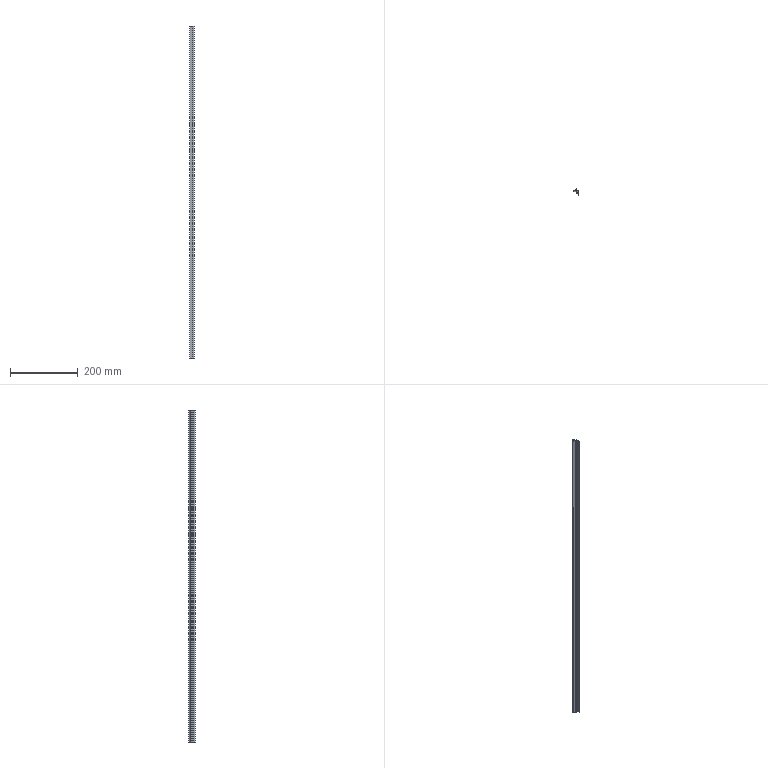Part | SolidWorks | features BaseBody 1, ICE 1, MoveFace 1 | 1 solid | 27 faces | box 14 x 20.3 x 980 mm | volume 49897 mm3 | plane 20 | cylinder 7 | commonest cylinder face diameters 0.387 x2 0.8 x2 0.4 x1 20 x1 22 x1
STEP:
#1=CARTESIAN_POINT('',(-5.304,-0.625,200.));
#2=VERTEX_POINT('',#1);
#3=CARTESIAN_POINT('',(-5.449,-0.8125,200.));
#4=VERTEX_POINT('',#3);
#5=CARTESIAN_POINT('',(-5.255,-0.8125,200.));
#6=DIRECTION('',(0.,0.,1.));
#7=DIRECTION('',(-1.,0.,0.));
#8=AXIS2_PLACEMENT_3D('',#5,#6,#7);
#9=CIRCLE('',#8,0.1937);
#10=EDGE_CURVE('',#2,#4,#9,.T.);
#11=ORIENTED_EDGE('',*,*,#10,.T.);
#12=CARTESIAN_POINT('',(-5.449,-0.8125,-780.));
#13=VERTEX_POINT('',#12);
#14=CARTESIAN_POINT('',(-5.449,-0.8125,230.));
#15=DIRECTION('',(0.,0.,-1.));
#16=VECTOR('',#15,1000.);
#17=LINE('',#14,#16);
#18=EDGE_CURVE('',#4,#13,#17,.T.);
#19=ORIENTED_EDGE('',*,*,#18,.T.);
#20=CARTESIAN_POINT('',(-5.304,-0.625,-780.));
#21=VERTEX_POINT('',#20);
#22=CARTESIAN_POINT('',(-5.255,-0.8125,-780.));
#23=DIRECTION('',(0.,0.,-1.));
#24=DIRECTION('',(1.,0.,0.));
#25=AXIS2_PLACEMENT_3D('',#22,#23,#24);
#26=CIRCLE('',#25,0.1937);
#27=EDGE_CURVE('',#13,#21,#26,.T.);
#28=ORIENTED_EDGE('',*,*,#27,.T.);
#29=CARTESIAN_POINT('',(-5.304,-0.625,230.));
#30=DIRECTION('',(0.,0.,-1.));
#31=VECTOR('',#30,1000.);
#32=LINE('',#29,#31);
#33=EDGE_CURVE('',#2,#21,#32,.T.);
#34=ORIENTED_EDGE('',*,*,#33,.F.);
#35=EDGE_LOOP('',(#11,#19,#28,#34));
#36=FACE_OUTER_BOUND('',#35,.T.);
#37=CARTESIAN_POINT('',(-5.255,-0.8125,230.));
#38=DIRECTION('',(0.,0.,-1.));
#39=DIRECTION('',(-1.,0.,0.));
#40=AXIS2_PLACEMENT_3D('',#37,#38,#39);
#41=CYLINDRICAL_SURFACE('',#40,0.1937);
#42=ADVANCED_FACE('',(#36),#41,.F.);
#43=CARTESIAN_POINT('',(5.,-1.,-780.));
#44=VERTEX_POINT('',#43);
#45=CARTESIAN_POINT('',(5.,-14.3,-780.));
#46=VERTEX_POINT('',#45);
#47=CARTESIAN_POINT('',(5.,29.623,-780.));
#48=DIRECTION('',(0.,-1.,0.));
#49=VECTOR('',#48,1000.);
#50=LINE('',#47,#49);
#51=EDGE_CURVE('',#44,#46,#50,.T.);
#52=ORIENTED_EDGE('',*,*,#51,.F.);
#53=CARTESIAN_POINT('',(5.,-1.,200.));
#54=VERTEX_POINT('',#53);
#55=CARTESIAN_POINT('',(5.,-1.,230.));
#56=DIRECTION('',(0.,0.,-1.));
#57=VECTOR('',#56,1000.);
#58=LINE('',#55,#57);
#59=EDGE_CURVE('',#54,#44,#58,.T.);
#60=ORIENTED_EDGE('',*,*,#59,.F.);
#61=CARTESIAN_POINT('',(5.,-14.3,200.));
#62=VERTEX_POINT('',#61);
#63=CARTESIAN_POINT('',(5.,-14.3,200.));
#64=DIRECTION('',(0.,1.,0.));
#65=VECTOR('',#64,1000.);
#66=LINE('',#63,#65);
#67=EDGE_CURVE('',#62,#54,#66,.T.);
#68=ORIENTED_EDGE('',*,*,#67,.F.);
#69=CARTESIAN_POINT('',(5.,-14.3,230.));
#70=DIRECTION('',(0.,0.,1.));
#71=VECTOR('',#70,1000.);
#72=LINE('',#69,#71);
#73=EDGE_CURVE('',#46,#62,#72,.T.);
#74=ORIENTED_EDGE('',*,*,#73,.F.);
#75=EDGE_LOOP('',(#52,#60,#68,#74));
#76=FACE_OUTER_BOUND('',#75,.T.);
#77=CARTESIAN_POINT('',(5.,-14.3,230.));
#78=DIRECTION('',(-1.,0.,0.));
#79=DIRECTION('',(0.,0.,1.));
#80=AXIS2_PLACEMENT_3D('',#77,#78,#79);
#81=PLANE('',#80);
#82=ADVANCED_FACE('',(#76),#81,.F.);
#83=CARTESIAN_POINT('',(-9.,-2.,-780.));
#84=VERTEX_POINT('',#83);
#85=CARTESIAN_POINT('',(-9.,-2.,200.));
#86=VERTEX_POINT('',#85);
#87=CARTESIAN_POINT('',(-9.,-2.,230.));
#88=DIRECTION('',(0.,0.,1.));
#89=VECTOR('',#88,1000.);
#90=LINE('',#87,#89);
#91=EDGE_CURVE('',#84,#86,#90,.T.);
#92=ORIENTED_EDGE('',*,*,#91,.F.);
#93=CARTESIAN_POINT('',(0.9,-2.,-780.));
#94=VERTEX_POINT('',#93);
#95=CARTESIAN_POINT('',(5.,-2.,-780.));
#96=DIRECTION('',(-1.,0.,0.));
#97=VECTOR('',#96,1000.);
#98=LINE('',#95,#97);
#99=EDGE_CURVE('',#94,#84,#98,.T.);
#100=ORIENTED_EDGE('',*,*,#99,.F.);
#101=CARTESIAN_POINT('',(0.9,-2.,200.));
#102=VERTEX_POINT('',#101);
#103=CARTESIAN_POINT('',(0.9,-2.,230.));
#104=DIRECTION('',(0.,0.,-1.));
#105=VECTOR('',#104,1000.);
#106=LINE('',#103,#105);
#107=EDGE_CURVE('',#102,#94,#106,.T.);
#108=ORIENTED_EDGE('',*,*,#107,.F.);
#109=CARTESIAN_POINT('',(5.,-2.,200.));
#110=DIRECTION('',(1.,0.,0.));
#111=VECTOR('',#110,1000.);
#112=LINE('',#109,#111);
#113=EDGE_CURVE('',#86,#102,#112,.T.);
#114=ORIENTED_EDGE('',*,*,#113,.F.);
#115=EDGE_LOOP('',(#92,#100,#108,#114));
#116=FACE_OUTER_BOUND('',#115,.T.);
#117=CARTESIAN_POINT('',(-9.,-2.,230.));
#118=DIRECTION('',(0.,1.,0.));
#119=DIRECTION('',(0.,0.,1.));
#120=AXIS2_PLACEMENT_3D('',#117,#118,#119);
#121=PLANE('',#120);
#122=ADVANCED_FACE('',(#116),#121,.F.);
#123=CARTESIAN_POINT('',(4.,-6.,200.));
#124=VERTEX_POINT('',#123);
#125=CARTESIAN_POINT('',(4.,-3.,200.));
#126=VERTEX_POINT('',#125);
#127=CARTESIAN_POINT('',(4.,29.623,200.));
#128=DIRECTION('',(0.,1.,0.));
#129=VECTOR('',#128,1000.);
#130=LINE('',#127,#129);
#131=EDGE_CURVE('',#124,#126,#130,.T.);
#132=ORIENTED_EDGE('',*,*,#131,.F.);
#133=CARTESIAN_POINT('',(1.,-6.,200.));
#134=VERTEX_POINT('',#133);
#135=CARTESIAN_POINT('',(5.,-6.,200.));
#136=DIRECTION('',(1.,0.,0.));
#137=VECTOR('',#136,1000.);
#138=LINE('',#135,#137);
#139=EDGE_CURVE('',#134,#124,#138,.T.);
#140=ORIENTED_EDGE('',*,*,#139,.F.);
#141=CARTESIAN_POINT('',(1.,-6.7,200.));
#142=VERTEX_POINT('',#141);
#143=CARTESIAN_POINT('',(1.,-6.,200.));
#144=DIRECTION('',(0.,-1.,0.));
#145=VECTOR('',#144,1000.);
#146=LINE('',#143,#145);
#147=EDGE_CURVE('',#134,#142,#146,.T.);
#148=ORIENTED_EDGE('',*,*,#147,.T.);
#149=CARTESIAN_POINT('',(-1.7,-6.7,200.));
#150=VERTEX_POINT('',#149);
#151=CARTESIAN_POINT('',(5.,-6.7,200.));
#152=DIRECTION('',(1.,0.,0.));
#153=VECTOR('',#152,1000.);
#154=LINE('',#151,#153);
#155=EDGE_CURVE('',#150,#142,#154,.T.);
#156=ORIENTED_EDGE('',*,*,#155,.F.);
#157=CARTESIAN_POINT('',(-1.7,-7.7,200.));
#158=VERTEX_POINT('',#157);
#159=CARTESIAN_POINT('',(-1.7,-6.7,200.));
#160=DIRECTION('',(0.,-1.,0.));
#161=VECTOR('',#160,1000.);
#162=LINE('',#159,#161);
#163=EDGE_CURVE('',#150,#158,#162,.T.);
#164=ORIENTED_EDGE('',*,*,#163,.T.);
#165=CARTESIAN_POINT('',(4.,-7.7,200.));
#166=VERTEX_POINT('',#165);
#167=CARTESIAN_POINT('',(5.,-7.7,200.));
#168=DIRECTION('',(-1.,0.,0.));
#169=VECTOR('',#168,1000.);
#170=LINE('',#167,#169);
#171=EDGE_CURVE('',#166,#158,#170,.T.);
#172=ORIENTED_EDGE('',*,*,#171,.F.);
#173=CARTESIAN_POINT('',(4.,-14.3,200.));
#174=VERTEX_POINT('',#173);
#175=CARTESIAN_POINT('',(4.,29.623,200.));
#176=DIRECTION('',(0.,1.,0.));
#177=VECTOR('',#176,1000.);
#178=LINE('',#175,#177);
#179=EDGE_CURVE('',#174,#166,#178,.T.);
#180=ORIENTED_EDGE('',*,*,#179,.F.);
#181=CARTESIAN_POINT('',(5.,-14.3,200.));
#182=DIRECTION('',(-1.,0.,0.));
#183=VECTOR('',#182,1000.);
#184=LINE('',#181,#183);
#185=EDGE_CURVE('',#62,#174,#184,.T.);
#186=ORIENTED_EDGE('',*,*,#185,.F.);
#187=ORIENTED_EDGE('',*,*,#67,.T.);
#188=CARTESIAN_POINT('',(-5.207,-1.,200.));
#189=VERTEX_POINT('',#188);
#190=CARTESIAN_POINT('',(5.,-1.,200.));
#191=DIRECTION('',(1.,0.,0.));
#192=VECTOR('',#191,1000.);
#193=LINE('',#190,#192);
#194=EDGE_CURVE('',#189,#54,#193,.T.);
#195=ORIENTED_EDGE('',*,*,#194,.F.);
#196=CARTESIAN_POINT('',(-5.255,-0.8125,200.));
#197=DIRECTION('',(0.,0.,1.));
#198=DIRECTION('',(-1.,0.,0.));
#199=AXIS2_PLACEMENT_3D('',#196,#197,#198);
#200=CIRCLE('',#199,0.1937);
#201=EDGE_CURVE('',#4,#189,#200,.T.);
#202=ORIENTED_EDGE('',*,*,#201,.F.);
#203=ORIENTED_EDGE('',*,*,#10,.F.);
#204=CARTESIAN_POINT('',(-1.368,3.063,200.));
#205=VERTEX_POINT('',#204);
#206=CARTESIAN_POINT('',(-10.628,9.,200.));
#207=DIRECTION('',(0.,0.,1.));
#208=DIRECTION('',(-1.,0.,0.));
#209=AXIS2_PLACEMENT_3D('',#206,#207,#208);
#210=CIRCLE('',#209,11.);
#211=EDGE_CURVE('',#2,#205,#210,.T.);
#212=ORIENTED_EDGE('',*,*,#211,.T.);
#213=CARTESIAN_POINT('',(-1.,2.955,200.));
#214=VERTEX_POINT('',#213);
#215=CARTESIAN_POINT('',(-1.2,2.955,200.));
#216=DIRECTION('',(0.,0.,1.));
#217=DIRECTION('',(-1.,0.,0.));
#218=AXIS2_PLACEMENT_3D('',#215,#216,#217);
#219=CIRCLE('',#218,0.2);
#220=EDGE_CURVE('',#214,#205,#219,.T.);
#221=ORIENTED_EDGE('',*,*,#220,.F.);
#222=CARTESIAN_POINT('',(-1.,1.5,200.));
#223=VERTEX_POINT('',#222);
#224=CARTESIAN_POINT('',(-1.,2.955,200.));
#225=DIRECTION('',(0.,1.,0.));
#226=VECTOR('',#225,1000.);
#227=LINE('',#224,#226);
#228=EDGE_CURVE('',#223,#214,#227,.T.);
#229=ORIENTED_EDGE('',*,*,#228,.F.);
#230=CARTESIAN_POINT('',(0.,1.5,200.));
#231=VERTEX_POINT('',#230);
#232=CARTESIAN_POINT('',(-1.,1.5,200.));
#233=DIRECTION('',(-1.,0.,0.));
#234=VECTOR('',#233,1000.);
#235=LINE('',#232,#234);
#236=EDGE_CURVE('',#231,#223,#235,.T.);
#237=ORIENTED_EDGE('',*,*,#236,.F.);
#238=CARTESIAN_POINT('',(0.,6.,200.));
#239=VERTEX_POINT('',#238);
#240=CARTESIAN_POINT('',(0.,1.5,200.));
#241=DIRECTION('',(0.,-1.,0.));
#242=VECTOR('',#241,1000.);
#243=LINE('',#240,#242);
#244=EDGE_CURVE('',#239,#231,#243,.T.);
#245=ORIENTED_EDGE('',*,*,#244,.F.);
#246=CARTESIAN_POINT('',(-0.8,6.,200.));
#247=VERTEX_POINT('',#246);
#248=CARTESIAN_POINT('',(0.,6.,200.));
#249=DIRECTION('',(1.,0.,0.));
#250=VECTOR('',#249,1000.);
#251=LINE('',#248,#250);
#252=EDGE_CURVE('',#247,#239,#251,.T.);
#253=ORIENTED_EDGE('',*,*,#252,.F.);
#254=CARTESIAN_POINT('',(-1.178,5.731,200.));
#255=VERTEX_POINT('',#254);
#256=CARTESIAN_POINT('',(-0.8,5.6,200.));
#257=DIRECTION('',(0.,0.,1.));
#258=DIRECTION('',(-1.,0.,0.));
#259=AXIS2_PLACEMENT_3D('',#256,#257,#258);
#260=CIRCLE('',#259,0.4);
#261=EDGE_CURVE('',#247,#255,#260,.T.);
#262=ORIENTED_EDGE('',*,*,#261,.T.);
#263=CARTESIAN_POINT('',(-8.678,-0.8077,200.));
#264=VERTEX_POINT('',#263);
#265=CARTESIAN_POINT('',(-10.628,9.,200.));
#266=DIRECTION('',(0.,0.,1.));
#267=DIRECTION('',(-1.,0.,0.));
#268=AXIS2_PLACEMENT_3D('',#265,#266,#267);
#269=CIRCLE('',#268,10.);
#270=EDGE_CURVE('',#264,#255,#269,.T.);
#271=ORIENTED_EDGE('',*,*,#270,.F.);
#272=CARTESIAN_POINT('',(-9.,-1.2,200.));
#273=VERTEX_POINT('',#272);
#274=CARTESIAN_POINT('',(-8.6,-1.2,200.));
#275=DIRECTION('',(0.,0.,1.));
#276=DIRECTION('',(-1.,0.,0.));
#277=AXIS2_PLACEMENT_3D('',#274,#275,#276);
#278=CIRCLE('',#277,0.4);
#279=EDGE_CURVE('',#264,#273,#278,.T.);
#280=ORIENTED_EDGE('',*,*,#279,.T.);
#281=CARTESIAN_POINT('',(-9.,8.,200.));
#282=DIRECTION('',(0.,-1.,0.));
#283=VECTOR('',#282,1000.);
#284=LINE('',#281,#283);
#285=EDGE_CURVE('',#273,#86,#284,.T.);
#286=ORIENTED_EDGE('',*,*,#285,.T.);
#287=ORIENTED_EDGE('',*,*,#113,.T.);
#288=CARTESIAN_POINT('',(0.9,-3.,200.));
#289=VERTEX_POINT('',#288);
#290=CARTESIAN_POINT('',(0.9,29.623,200.));
#291=DIRECTION('',(0.,1.,0.));
#292=VECTOR('',#291,1000.);
#293=LINE('',#290,#292);
#294=EDGE_CURVE('',#289,#102,#293,.T.);
#295=ORIENTED_EDGE('',*,*,#294,.F.);
#296=CARTESIAN_POINT('',(5.,-3.,200.));
#297=DIRECTION('',(-1.,0.,0.));
#298=VECTOR('',#297,1000.);
#299=LINE('',#296,#298);
#300=EDGE_CURVE('',#126,#289,#299,.T.);
#301=ORIENTED_EDGE('',*,*,#300,.F.);
#302=EDGE_LOOP('',(#132,#140,#148,#156,#164,#172,#180,#186,#187,#195,#202,#203,#212,#221,#229,#237,#245,#253,#262,#271,#280,#286,#287,#295,#301));
#303=FACE_OUTER_BOUND('',#302,.T.);
#304=CARTESIAN_POINT('',(5.,29.623,200.));
#305=DIRECTION('',(0.,0.,-1.));
#306=DIRECTION('',(-1.,0.,0.));
#307=AXIS2_PLACEMENT_3D('',#304,#305,#306);
#308=PLANE('',#307);
#309=ADVANCED_FACE('',(#303),#308,.F.);
#310=ORIENTED_EDGE('',*,*,#185,.T.);
#311=CARTESIAN_POINT('',(4.,-14.3,-780.));
#312=VERTEX_POINT('',#311);
#313=CARTESIAN_POINT('',(4.,-14.3,230.));
#314=DIRECTION('',(0.,0.,1.));
#315=VECTOR('',#314,1000.);
#316=LINE('',#313,#315);
#317=EDGE_CURVE('',#312,#174,#316,.T.);
#318=ORIENTED_EDGE('',*,*,#317,.F.);
#319=CARTESIAN_POINT('',(5.,-14.3,-780.));
#320=DIRECTION('',(-1.,0.,0.));
#321=VECTOR('',#320,1000.);
#322=LINE('',#319,#321);
#323=EDGE_CURVE('',#46,#312,#322,.T.);
#324=ORIENTED_EDGE('',*,*,#323,.F.);
#325=ORIENTED_EDGE('',*,*,#73,.T.);
#326=EDGE_LOOP('',(#310,#318,#324,#325));
#327=FACE_OUTER_BOUND('',#326,.T.);
#328=CARTESIAN_POINT('',(4.,-14.3,230.));
#329=DIRECTION('',(0.,1.,0.));
#330=DIRECTION('',(0.,0.,1.));
#331=AXIS2_PLACEMENT_3D('',#328,#329,#330);
#332=PLANE('',#331);
#333=ADVANCED_FACE('',(#327),#332,.F.);
#334=ORIENTED_EDGE('',*,*,#51,.T.);
#335=ORIENTED_EDGE('',*,*,#323,.T.);
#336=CARTESIAN_POINT('',(4.,-7.7,-780.));
#337=VERTEX_POINT('',#336);
#338=CARTESIAN_POINT('',(4.,-7.7,-780.));
#339=DIRECTION('',(0.,-1.,0.));
#340=VECTOR('',#339,1000.);
#341=LINE('',#338,#340);
#342=EDGE_CURVE('',#337,#312,#341,.T.);
#343=ORIENTED_EDGE('',*,*,#342,.F.);
#344=CARTESIAN_POINT('',(-1.7,-7.7,-780.));
#345=VERTEX_POINT('',#344);
#346=CARTESIAN_POINT('',(-1.7,-7.7,-780.));
#347=DIRECTION('',(1.,0.,0.));
#348=VECTOR('',#347,1000.);
#349=LINE('',#346,#348);
#350=EDGE_CURVE('',#345,#337,#349,.T.);
#351=ORIENTED_EDGE('',*,*,#350,.F.);
#352=CARTESIAN_POINT('',(-1.7,-6.7,-780.));
#353=VERTEX_POINT('',#352);
#354=CARTESIAN_POINT('',(-1.7,29.623,-780.));
#355=DIRECTION('',(0.,1.,0.));
#356=VECTOR('',#355,1000.);
#357=LINE('',#354,#356);
#358=EDGE_CURVE('',#345,#353,#357,.T.);
#359=ORIENTED_EDGE('',*,*,#358,.T.);
#360=CARTESIAN_POINT('',(1.,-6.7,-780.));
#361=VERTEX_POINT('',#360);
#362=CARTESIAN_POINT('',(1.,-6.7,-780.));
#363=DIRECTION('',(-1.,0.,0.));
#364=VECTOR('',#363,1000.);
#365=LINE('',#362,#364);
#366=EDGE_CURVE('',#361,#353,#365,.T.);
#367=ORIENTED_EDGE('',*,*,#366,.F.);
#368=CARTESIAN_POINT('',(1.,-6.,-780.));
#369=VERTEX_POINT('',#368);
#370=CARTESIAN_POINT('',(1.,29.623,-780.));
#371=DIRECTION('',(0.,1.,0.));
#372=VECTOR('',#371,1000.);
#373=LINE('',#370,#372);
#374=EDGE_CURVE('',#361,#369,#373,.T.);
#375=ORIENTED_EDGE('',*,*,#374,.T.);
#376=CARTESIAN_POINT('',(4.,-6.,-780.));
#377=VERTEX_POINT('',#376);
#378=CARTESIAN_POINT('',(4.,-6.,-780.));
#379=DIRECTION('',(-1.,0.,0.));
#380=VECTOR('',#379,1000.);
#381=LINE('',#378,#380);
#382=EDGE_CURVE('',#377,#369,#381,.T.);
#383=ORIENTED_EDGE('',*,*,#382,.F.);
#384=CARTESIAN_POINT('',(4.,-3.,-780.));
#385=VERTEX_POINT('',#384);
#386=CARTESIAN_POINT('',(4.,-3.,-780.));
#387=DIRECTION('',(0.,-1.,0.));
#388=VECTOR('',#387,1000.);
#389=LINE('',#386,#388);
#390=EDGE_CURVE('',#385,#377,#389,.T.);
#391=ORIENTED_EDGE('',*,*,#390,.F.);
#392=CARTESIAN_POINT('',(0.9,-3.,-780.));
#393=VERTEX_POINT('',#392);
#394=CARTESIAN_POINT('',(0.9,-3.,-780.));
#395=DIRECTION('',(1.,0.,0.));
#396=VECTOR('',#395,1000.);
#397=LINE('',#394,#396);
#398=EDGE_CURVE('',#393,#385,#397,.T.);
#399=ORIENTED_EDGE('',*,*,#398,.F.);
#400=CARTESIAN_POINT('',(0.9,-2.,-780.));
#401=DIRECTION('',(0.,-1.,0.));
#402=VECTOR('',#401,1000.);
#403=LINE('',#400,#402);
#404=EDGE_CURVE('',#94,#393,#403,.T.);
#405=ORIENTED_EDGE('',*,*,#404,.F.);
#406=ORIENTED_EDGE('',*,*,#99,.T.);
#407=CARTESIAN_POINT('',(-9.,-1.2,-780.));
#408=VERTEX_POINT('',#407);
#409=CARTESIAN_POINT('',(-9.,-1.2,-780.));
#410=DIRECTION('',(0.,-1.,0.));
#411=VECTOR('',#410,1000.);
#412=LINE('',#409,#411);
#413=EDGE_CURVE('',#408,#84,#412,.T.);
#414=ORIENTED_EDGE('',*,*,#413,.F.);
#415=CARTESIAN_POINT('',(-8.678,-0.8077,-780.));
#416=VERTEX_POINT('',#415);
#417=CARTESIAN_POINT('',(-8.6,-1.2,-780.));
#418=DIRECTION('',(0.,0.,-1.));
#419=DIRECTION('',(1.,0.,0.));
#420=AXIS2_PLACEMENT_3D('',#417,#418,#419);
#421=CIRCLE('',#420,0.4);
#422=EDGE_CURVE('',#408,#416,#421,.T.);
#423=ORIENTED_EDGE('',*,*,#422,.T.);
#424=CARTESIAN_POINT('',(-1.178,5.731,-780.));
#425=VERTEX_POINT('',#424);
#426=CARTESIAN_POINT('',(-10.628,9.,-780.));
#427=DIRECTION('',(0.,0.,-1.));
#428=DIRECTION('',(1.,0.,0.));
#429=AXIS2_PLACEMENT_3D('',#426,#427,#428);
#430=CIRCLE('',#429,10.);
#431=EDGE_CURVE('',#425,#416,#430,.T.);
#432=ORIENTED_EDGE('',*,*,#431,.F.);
#433=CARTESIAN_POINT('',(-0.8,6.,-780.));
#434=VERTEX_POINT('',#433);
#435=CARTESIAN_POINT('',(-0.8,5.6,-780.));
#436=DIRECTION('',(0.,0.,-1.));
#437=DIRECTION('',(1.,0.,0.));
#438=AXIS2_PLACEMENT_3D('',#435,#436,#437);
#439=CIRCLE('',#438,0.4);
#440=EDGE_CURVE('',#425,#434,#439,.T.);
#441=ORIENTED_EDGE('',*,*,#440,.T.);
#442=CARTESIAN_POINT('',(0.,6.,-780.));
#443=VERTEX_POINT('',#442);
#444=CARTESIAN_POINT('',(0.,6.,-780.));
#445=DIRECTION('',(-1.,0.,0.));
#446=VECTOR('',#445,1000.);
#447=LINE('',#444,#446);
#448=EDGE_CURVE('',#443,#434,#447,.T.);
#449=ORIENTED_EDGE('',*,*,#448,.F.);
#450=CARTESIAN_POINT('',(0.,1.5,-780.));
#451=VERTEX_POINT('',#450);
#452=CARTESIAN_POINT('',(0.,1.5,-780.));
#453=DIRECTION('',(0.,1.,0.));
#454=VECTOR('',#453,1000.);
#455=LINE('',#452,#454);
#456=EDGE_CURVE('',#451,#443,#455,.T.);
#457=ORIENTED_EDGE('',*,*,#456,.F.);
#458=CARTESIAN_POINT('',(-1.,1.5,-780.));
#459=VERTEX_POINT('',#458);
#460=CARTESIAN_POINT('',(-1.,1.5,-780.));
#461=DIRECTION('',(1.,0.,0.));
#462=VECTOR('',#461,1000.);
#463=LINE('',#460,#462);
#464=EDGE_CURVE('',#459,#451,#463,.T.);
#465=ORIENTED_EDGE('',*,*,#464,.F.);
#466=CARTESIAN_POINT('',(-1.,2.955,-780.));
#467=VERTEX_POINT('',#466);
#468=CARTESIAN_POINT('',(-1.,2.955,-780.));
#469=DIRECTION('',(0.,-1.,0.));
#470=VECTOR('',#469,1000.);
#471=LINE('',#468,#470);
#472=EDGE_CURVE('',#467,#459,#471,.T.);
#473=ORIENTED_EDGE('',*,*,#472,.F.);
#474=CARTESIAN_POINT('',(-1.368,3.063,-780.));
#475=VERTEX_POINT('',#474);
#476=CARTESIAN_POINT('',(-1.2,2.955,-780.));
#477=DIRECTION('',(0.,0.,-1.));
#478=DIRECTION('',(1.,0.,0.));
#479=AXIS2_PLACEMENT_3D('',#476,#477,#478);
#480=CIRCLE('',#479,0.2);
#481=EDGE_CURVE('',#475,#467,#480,.T.);
#482=ORIENTED_EDGE('',*,*,#481,.F.);
#483=CARTESIAN_POINT('',(-10.628,9.,-780.));
#484=DIRECTION('',(0.,0.,-1.));
#485=DIRECTION('',(1.,0.,0.));
#486=AXIS2_PLACEMENT_3D('',#483,#484,#485);
#487=CIRCLE('',#486,11.);
#488=EDGE_CURVE('',#475,#21,#487,.T.);
#489=ORIENTED_EDGE('',*,*,#488,.T.);
#490=ORIENTED_EDGE('',*,*,#27,.F.);
#491=CARTESIAN_POINT('',(-5.207,-1.,-780.));
#492=VERTEX_POINT('',#491);
#493=CARTESIAN_POINT('',(-5.255,-0.8125,-780.));
#494=DIRECTION('',(0.,0.,-1.));
#495=DIRECTION('',(1.,0.,0.));
#496=AXIS2_PLACEMENT_3D('',#493,#494,#495);
#497=CIRCLE('',#496,0.1937);
#498=EDGE_CURVE('',#492,#13,#497,.T.);
#499=ORIENTED_EDGE('',*,*,#498,.F.);
#500=CARTESIAN_POINT('',(5.,-1.,-780.));
#501=DIRECTION('',(-1.,0.,0.));
#502=VECTOR('',#501,1000.);
#503=LINE('',#500,#502);
#504=EDGE_CURVE('',#44,#492,#503,.T.);
#505=ORIENTED_EDGE('',*,*,#504,.F.);
#506=EDGE_LOOP('',(#334,#335,#343,#351,#359,#367,#375,#383,#391,#399,#405,#406,#414,#423,#432,#441,#449,#457,#465,#473,#482,#489,#490,#499,#505));
#507=FACE_OUTER_BOUND('',#506,.T.);
#508=CARTESIAN_POINT('',(5.,29.623,-780.));
#509=DIRECTION('',(0.,0.,1.));
#510=DIRECTION('',(1.,0.,0.));
#511=AXIS2_PLACEMENT_3D('',#508,#509,#510);
#512=PLANE('',#511);
#513=ADVANCED_FACE('',(#507),#512,.F.);
#514=ORIENTED_EDGE('',*,*,#59,.T.);
#515=ORIENTED_EDGE('',*,*,#504,.T.);
#516=CARTESIAN_POINT('',(-5.207,-1.,230.));
#517=DIRECTION('',(0.,0.,-1.));
#518=VECTOR('',#517,1000.);
#519=LINE('',#516,#518);
#520=EDGE_CURVE('',#189,#492,#519,.T.);
#521=ORIENTED_EDGE('',*,*,#520,.F.);
#522=ORIENTED_EDGE('',*,*,#194,.T.);
#523=EDGE_LOOP('',(#514,#515,#521,#522));
#524=FACE_OUTER_BOUND('',#523,.T.);
#525=CARTESIAN_POINT('',(5.,-1.,230.));
#526=DIRECTION('',(0.,-1.,0.));
#527=DIRECTION('',(0.,0.,-1.));
#528=AXIS2_PLACEMENT_3D('',#525,#526,#527);
#529=PLANE('',#528);
#530=ADVANCED_FACE('',(#524),#529,.F.);
#531=CARTESIAN_POINT('',(-9.,-1.2,230.));
#532=DIRECTION('',(0.,0.,1.));
#533=VECTOR('',#532,1000.);
#534=LINE('',#531,#533);
#535=EDGE_CURVE('',#408,#273,#534,.T.);
#536=ORIENTED_EDGE('',*,*,#535,.F.);
#537=ORIENTED_EDGE('',*,*,#413,.T.);
#538=ORIENTED_EDGE('',*,*,#91,.T.);
#539=ORIENTED_EDGE('',*,*,#285,.F.);
#540=EDGE_LOOP('',(#536,#537,#538,#539));
#541=FACE_OUTER_BOUND('',#540,.T.);
#542=CARTESIAN_POINT('',(-9.,-1.2,230.));
#543=DIRECTION('',(1.,0.,0.));
#544=DIRECTION('',(0.,0.,-1.));
#545=AXIS2_PLACEMENT_3D('',#542,#543,#544);
#546=PLANE('',#545);
#547=ADVANCED_FACE('',(#541),#546,.F.);
#548=ORIENTED_EDGE('',*,*,#294,.T.);
#549=ORIENTED_EDGE('',*,*,#107,.T.);
#550=ORIENTED_EDGE('',*,*,#404,.T.);
#551=CARTESIAN_POINT('',(0.9,-3.,230.));
#552=DIRECTION('',(0.,0.,-1.));
#553=VECTOR('',#552,1000.);
#554=LINE('',#551,#553);
#555=EDGE_CURVE('',#289,#393,#554,.T.);
#556=ORIENTED_EDGE('',*,*,#555,.F.);
#557=EDGE_LOOP('',(#548,#549,#550,#556));
#558=FACE_OUTER_BOUND('',#557,.T.);
#559=CARTESIAN_POINT('',(0.9,-2.,230.));
#560=DIRECTION('',(1.,0.,0.));
#561=DIRECTION('',(0.,0.,-1.));
#562=AXIS2_PLACEMENT_3D('',#559,#560,#561);
#563=PLANE('',#562);
#564=ADVANCED_FACE('',(#558),#563,.F.);
#565=ORIENTED_EDGE('',*,*,#300,.T.);
#566=ORIENTED_EDGE('',*,*,#555,.T.);
#567=ORIENTED_EDGE('',*,*,#398,.T.);
#568=CARTESIAN_POINT('',(4.,-3.,230.));
#569=DIRECTION('',(0.,0.,-1.));
#570=VECTOR('',#569,1000.);
#571=LINE('',#568,#570);
#572=EDGE_CURVE('',#126,#385,#571,.T.);
#573=ORIENTED_EDGE('',*,*,#572,.F.);
#574=EDGE_LOOP('',(#565,#566,#567,#573));
#575=FACE_OUTER_BOUND('',#574,.T.);
#576=CARTESIAN_POINT('',(0.9,-3.,230.));
#577=DIRECTION('',(0.,1.,0.));
#578=DIRECTION('',(0.,0.,1.));
#579=AXIS2_PLACEMENT_3D('',#576,#577,#578);
#580=PLANE('',#579);
#581=ADVANCED_FACE('',(#575),#580,.F.);
#582=ORIENTED_EDGE('',*,*,#131,.T.);
#583=ORIENTED_EDGE('',*,*,#572,.T.);
#584=ORIENTED_EDGE('',*,*,#390,.T.);
#585=CARTESIAN_POINT('',(4.,-6.,230.));
#586=DIRECTION('',(0.,0.,-1.));
#587=VECTOR('',#586,1000.);
#588=LINE('',#585,#587);
#589=EDGE_CURVE('',#124,#377,#588,.T.);
#590=ORIENTED_EDGE('',*,*,#589,.F.);
#591=EDGE_LOOP('',(#582,#583,#584,#590));
#592=FACE_OUTER_BOUND('',#591,.T.);
#593=CARTESIAN_POINT('',(4.,-3.,230.));
#594=DIRECTION('',(1.,0.,0.));
#595=DIRECTION('',(0.,0.,-1.));
#596=AXIS2_PLACEMENT_3D('',#593,#594,#595);
#597=PLANE('',#596);
#598=ADVANCED_FACE('',(#592),#597,.F.);
#599=ORIENTED_EDGE('',*,*,#139,.T.);
#600=ORIENTED_EDGE('',*,*,#589,.T.);
#601=ORIENTED_EDGE('',*,*,#382,.T.);
#602=CARTESIAN_POINT('',(1.,-6.,230.));
#603=DIRECTION('',(0.,0.,-1.));
#604=VECTOR('',#603,1000.);
#605=LINE('',#602,#604);
#606=EDGE_CURVE('',#134,#369,#605,.T.);
#607=ORIENTED_EDGE('',*,*,#606,.F.);
#608=EDGE_LOOP('',(#599,#600,#601,#607));
#609=FACE_OUTER_BOUND('',#608,.T.);
#610=CARTESIAN_POINT('',(4.,-6.,230.));
#611=DIRECTION('',(0.,-1.,0.));
#612=DIRECTION('',(0.,0.,-1.));
#613=AXIS2_PLACEMENT_3D('',#610,#611,#612);
#614=PLANE('',#613);
#615=ADVANCED_FACE('',(#609),#614,.F.);
#616=ORIENTED_EDGE('',*,*,#155,.T.);
#617=CARTESIAN_POINT('',(1.,-6.7,230.));
#618=DIRECTION('',(0.,0.,1.));
#619=VECTOR('',#618,1000.);
#620=LINE('',#617,#619);
#621=EDGE_CURVE('',#361,#142,#620,.T.);
#622=ORIENTED_EDGE('',*,*,#621,.F.);
#623=ORIENTED_EDGE('',*,*,#366,.T.);
#624=CARTESIAN_POINT('',(-1.7,-6.7,230.));
#625=DIRECTION('',(0.,0.,-1.));
#626=VECTOR('',#625,1000.);
#627=LINE('',#624,#626);
#628=EDGE_CURVE('',#150,#353,#627,.T.);
#629=ORIENTED_EDGE('',*,*,#628,.F.);
#630=EDGE_LOOP('',(#616,#622,#623,#629));
#631=FACE_OUTER_BOUND('',#630,.T.);
#632=CARTESIAN_POINT('',(1.,-6.7,230.));
#633=DIRECTION('',(0.,-1.,0.));
#634=DIRECTION('',(0.,0.,-1.));
#635=AXIS2_PLACEMENT_3D('',#632,#633,#634);
#636=PLANE('',#635);
#637=ADVANCED_FACE('',(#631),#636,.F.);
#638=ORIENTED_EDGE('',*,*,#171,.T.);
#639=CARTESIAN_POINT('',(-1.7,-7.7,230.));
#640=DIRECTION('',(0.,0.,1.));
#641=VECTOR('',#640,1000.);
#642=LINE('',#639,#641);
#643=EDGE_CURVE('',#345,#158,#642,.T.);
#644=ORIENTED_EDGE('',*,*,#643,.F.);
#645=ORIENTED_EDGE('',*,*,#350,.T.);
#646=CARTESIAN_POINT('',(4.,-7.7,230.));
#647=DIRECTION('',(0.,0.,-1.));
#648=VECTOR('',#647,1000.);
#649=LINE('',#646,#648);
#650=EDGE_CURVE('',#166,#337,#649,.T.);
#651=ORIENTED_EDGE('',*,*,#650,.F.);
#652=EDGE_LOOP('',(#638,#644,#645,#651));
#653=FACE_OUTER_BOUND('',#652,.T.);
#654=CARTESIAN_POINT('',(-1.7,-7.7,230.));
#655=DIRECTION('',(0.,1.,0.));
#656=DIRECTION('',(0.,0.,1.));
#657=AXIS2_PLACEMENT_3D('',#654,#655,#656);
#658=PLANE('',#657);
#659=ADVANCED_FACE('',(#653),#658,.F.);
#660=ORIENTED_EDGE('',*,*,#179,.T.);
#661=ORIENTED_EDGE('',*,*,#650,.T.);
#662=ORIENTED_EDGE('',*,*,#342,.T.);
#663=ORIENTED_EDGE('',*,*,#317,.T.);
#664=EDGE_LOOP('',(#660,#661,#662,#663));
#665=FACE_OUTER_BOUND('',#664,.T.);
#666=CARTESIAN_POINT('',(4.,-7.7,230.));
#667=DIRECTION('',(1.,0.,0.));
#668=DIRECTION('',(0.,0.,-1.));
#669=AXIS2_PLACEMENT_3D('',#666,#667,#668);
#670=PLANE('',#669);
#671=ADVANCED_FACE('',(#665),#670,.F.);
#672=ORIENTED_EDGE('',*,*,#18,.F.);
#673=ORIENTED_EDGE('',*,*,#201,.T.);
#674=ORIENTED_EDGE('',*,*,#520,.T.);
#675=ORIENTED_EDGE('',*,*,#498,.T.);
#676=EDGE_LOOP('',(#672,#673,#674,#675));
#677=FACE_OUTER_BOUND('',#676,.T.);
#678=CARTESIAN_POINT('',(-5.255,-0.8125,230.));
#679=DIRECTION('',(0.,0.,-1.));
#680=DIRECTION('',(-1.,0.,0.));
#681=AXIS2_PLACEMENT_3D('',#678,#679,#680);
#682=CYLINDRICAL_SURFACE('',#681,0.1937);
#683=ADVANCED_FACE('',(#677),#682,.F.);
#684=CARTESIAN_POINT('',(-1.,2.955,230.));
#685=DIRECTION('',(0.,0.,1.));
#686=VECTOR('',#685,1000.);
#687=LINE('',#684,#686);
#688=EDGE_CURVE('',#467,#214,#687,.T.);
#689=ORIENTED_EDGE('',*,*,#688,.F.);
#690=ORIENTED_EDGE('',*,*,#472,.T.);
#691=CARTESIAN_POINT('',(-1.,1.5,230.));
#692=DIRECTION('',(0.,0.,-1.));
#693=VECTOR('',#692,1000.);
#694=LINE('',#691,#693);
#695=EDGE_CURVE('',#223,#459,#694,.T.);
#696=ORIENTED_EDGE('',*,*,#695,.F.);
#697=ORIENTED_EDGE('',*,*,#228,.T.);
#698=EDGE_LOOP('',(#689,#690,#696,#697));
#699=FACE_OUTER_BOUND('',#698,.T.);
#700=CARTESIAN_POINT('',(-1.,2.955,230.));
#701=DIRECTION('',(1.,0.,0.));
#702=DIRECTION('',(0.,0.,-1.));
#703=AXIS2_PLACEMENT_3D('',#700,#701,#702);
#704=PLANE('',#703);
#705=ADVANCED_FACE('',(#699),#704,.F.);
#706=ORIENTED_EDGE('',*,*,#488,.F.);
#707=CARTESIAN_POINT('',(-1.368,3.063,230.));
#708=DIRECTION('',(0.,0.,1.));
#709=VECTOR('',#708,1000.);
#710=LINE('',#707,#709);
#711=EDGE_CURVE('',#475,#205,#710,.T.);
#712=ORIENTED_EDGE('',*,*,#711,.T.);
#713=ORIENTED_EDGE('',*,*,#211,.F.);
#714=ORIENTED_EDGE('',*,*,#33,.T.);
#715=EDGE_LOOP('',(#706,#712,#713,#714));
#716=FACE_OUTER_BOUND('',#715,.T.);
#717=CARTESIAN_POINT('',(-10.628,9.,230.));
#718=DIRECTION('',(0.,0.,-1.));
#719=DIRECTION('',(-1.,0.,0.));
#720=AXIS2_PLACEMENT_3D('',#717,#718,#719);
#721=CYLINDRICAL_SURFACE('',#720,11.);
#722=ADVANCED_FACE('',(#716),#721,.T.);
#723=CARTESIAN_POINT('',(-1.178,5.731,230.));
#724=DIRECTION('',(0.,0.,1.));
#725=VECTOR('',#724,1000.);
#726=LINE('',#723,#725);
#727=EDGE_CURVE('',#425,#255,#726,.T.);
#728=ORIENTED_EDGE('',*,*,#727,.F.);
#729=ORIENTED_EDGE('',*,*,#431,.T.);
#730=CARTESIAN_POINT('',(-8.678,-0.8077,230.));
#731=DIRECTION('',(0.,0.,-1.));
#732=VECTOR('',#731,1000.);
#733=LINE('',#730,#732);
#734=EDGE_CURVE('',#264,#416,#733,.T.);
#735=ORIENTED_EDGE('',*,*,#734,.F.);
#736=ORIENTED_EDGE('',*,*,#270,.T.);
#737=EDGE_LOOP('',(#728,#729,#735,#736));
#738=FACE_OUTER_BOUND('',#737,.T.);
#739=CARTESIAN_POINT('',(-10.628,9.,230.));
#740=DIRECTION('',(0.,0.,-1.));
#741=DIRECTION('',(-1.,0.,0.));
#742=AXIS2_PLACEMENT_3D('',#739,#740,#741);
#743=CYLINDRICAL_SURFACE('',#742,10.);
#744=ADVANCED_FACE('',(#738),#743,.F.);
#745=CARTESIAN_POINT('',(0.,1.5,230.));
#746=DIRECTION('',(0.,0.,1.));
#747=VECTOR('',#746,1000.);
#748=LINE('',#745,#747);
#749=EDGE_CURVE('',#451,#231,#748,.T.);
#750=ORIENTED_EDGE('',*,*,#749,.F.);
#751=ORIENTED_EDGE('',*,*,#456,.T.);
#752=CARTESIAN_POINT('',(0.,6.,230.));
#753=DIRECTION('',(0.,0.,-1.));
#754=VECTOR('',#753,1000.);
#755=LINE('',#752,#754);
#756=EDGE_CURVE('',#239,#443,#755,.T.);
#757=ORIENTED_EDGE('',*,*,#756,.F.);
#758=ORIENTED_EDGE('',*,*,#244,.T.);
#759=EDGE_LOOP('',(#750,#751,#757,#758));
#760=FACE_OUTER_BOUND('',#759,.T.);
#761=CARTESIAN_POINT('',(0.,1.5,230.));
#762=DIRECTION('',(-1.,0.,0.));
#763=DIRECTION('',(0.,0.,1.));
#764=AXIS2_PLACEMENT_3D('',#761,#762,#763);
#765=PLANE('',#764);
#766=ADVANCED_FACE('',(#760),#765,.F.);
#767=ORIENTED_EDGE('',*,*,#422,.F.);
#768=ORIENTED_EDGE('',*,*,#535,.T.);
#769=ORIENTED_EDGE('',*,*,#279,.F.);
#770=ORIENTED_EDGE('',*,*,#734,.T.);
#771=EDGE_LOOP('',(#767,#768,#769,#770));
#772=FACE_OUTER_BOUND('',#771,.T.);
#773=CARTESIAN_POINT('',(-8.6,-1.2,230.));
#774=DIRECTION('',(0.,0.,-1.));
#775=DIRECTION('',(-1.,0.,0.));
#776=AXIS2_PLACEMENT_3D('',#773,#774,#775);
#777=CYLINDRICAL_SURFACE('',#776,0.4);
#778=ADVANCED_FACE('',(#772),#777,.T.);
#779=ORIENTED_EDGE('',*,*,#147,.F.);
#780=ORIENTED_EDGE('',*,*,#606,.T.);
#781=ORIENTED_EDGE('',*,*,#374,.F.);
#782=ORIENTED_EDGE('',*,*,#621,.T.);
#783=EDGE_LOOP('',(#779,#780,#781,#782));
#784=FACE_OUTER_BOUND('',#783,.T.);
#785=CARTESIAN_POINT('',(1.,-6.,230.));
#786=DIRECTION('',(1.,0.,0.));
#787=DIRECTION('',(0.,0.,-1.));
#788=AXIS2_PLACEMENT_3D('',#785,#786,#787);
#789=PLANE('',#788);
#790=ADVANCED_FACE('',(#784),#789,.F.);
#791=ORIENTED_EDGE('',*,*,#163,.F.);
#792=ORIENTED_EDGE('',*,*,#628,.T.);
#793=ORIENTED_EDGE('',*,*,#358,.F.);
#794=ORIENTED_EDGE('',*,*,#643,.T.);
#795=EDGE_LOOP('',(#791,#792,#793,#794));
#796=FACE_OUTER_BOUND('',#795,.T.);
#797=CARTESIAN_POINT('',(-1.7,-6.7,230.));
#798=DIRECTION('',(1.,0.,0.));
#799=DIRECTION('',(0.,0.,-1.));
#800=AXIS2_PLACEMENT_3D('',#797,#798,#799);
#801=PLANE('',#800);
#802=ADVANCED_FACE('',(#796),#801,.F.);
#803=ORIENTED_EDGE('',*,*,#711,.F.);
#804=ORIENTED_EDGE('',*,*,#481,.T.);
#805=ORIENTED_EDGE('',*,*,#688,.T.);
#806=ORIENTED_EDGE('',*,*,#220,.T.);
#807=EDGE_LOOP('',(#803,#804,#805,#806));
#808=FACE_OUTER_BOUND('',#807,.T.);
#809=CARTESIAN_POINT('',(-1.2,2.955,230.));
#810=DIRECTION('',(0.,0.,-1.));
#811=DIRECTION('',(-1.,0.,0.));
#812=AXIS2_PLACEMENT_3D('',#809,#810,#811);
#813=CYLINDRICAL_SURFACE('',#812,0.2);
#814=ADVANCED_FACE('',(#808),#813,.F.);
#815=ORIENTED_EDGE('',*,*,#695,.T.);
#816=ORIENTED_EDGE('',*,*,#464,.T.);
#817=ORIENTED_EDGE('',*,*,#749,.T.);
#818=ORIENTED_EDGE('',*,*,#236,.T.);
#819=EDGE_LOOP('',(#815,#816,#817,#818));
#820=FACE_OUTER_BOUND('',#819,.T.);
#821=CARTESIAN_POINT('',(-1.,1.5,230.));
#822=DIRECTION('',(0.,1.,0.));
#823=DIRECTION('',(0.,0.,1.));
#824=AXIS2_PLACEMENT_3D('',#821,#822,#823);
#825=PLANE('',#824);
#826=ADVANCED_FACE('',(#820),#825,.F.);
#827=ORIENTED_EDGE('',*,*,#440,.F.);
#828=ORIENTED_EDGE('',*,*,#727,.T.);
#829=ORIENTED_EDGE('',*,*,#261,.F.);
#830=CARTESIAN_POINT('',(-0.8,6.,230.));
#831=DIRECTION('',(0.,0.,-1.));
#832=VECTOR('',#831,1000.);
#833=LINE('',#830,#832);
#834=EDGE_CURVE('',#247,#434,#833,.T.);
#835=ORIENTED_EDGE('',*,*,#834,.T.);
#836=EDGE_LOOP('',(#827,#828,#829,#835));
#837=FACE_OUTER_BOUND('',#836,.T.);
#838=CARTESIAN_POINT('',(-0.8,5.6,230.));
#839=DIRECTION('',(0.,0.,-1.));
#840=DIRECTION('',(-1.,0.,0.));
#841=AXIS2_PLACEMENT_3D('',#838,#839,#840);
#842=CYLINDRICAL_SURFACE('',#841,0.4);
#843=ADVANCED_FACE('',(#837),#842,.T.);
#844=ORIENTED_EDGE('',*,*,#756,.T.);
#845=ORIENTED_EDGE('',*,*,#448,.T.);
#846=ORIENTED_EDGE('',*,*,#834,.F.);
#847=ORIENTED_EDGE('',*,*,#252,.T.);
#848=EDGE_LOOP('',(#844,#845,#846,#847));
#849=FACE_OUTER_BOUND('',#848,.T.);
#850=CARTESIAN_POINT('',(0.,6.,230.));
#851=DIRECTION('',(0.,-1.,0.));
#852=DIRECTION('',(0.,0.,-1.));
#853=AXIS2_PLACEMENT_3D('',#850,#851,#852);
#854=PLANE('',#853);
#855=ADVANCED_FACE('',(#849),#854,.F.);
#856=CLOSED_SHELL('',(#42,#82,#122,#309,#333,#513,#530,#547,#564,#581,#598,#615,#637,#659,#671,#683,#705,#722,#744,#766,#778,#790,#802,#814,#826,#843,#855));
#857=MANIFOLD_SOLID_BREP('',#856);
#858=CARTESIAN_POINT('',(0.,0.,0.));
#859=DIRECTION('',(0.,0.,1.));
#860=DIRECTION('',(1.,0.,0.));
#861=AXIS2_PLACEMENT_3D('',#858,#859,#860);
#862=(LENGTH_UNIT()NAMED_UNIT(*)SI_UNIT(.MILLI.,.METRE.));
#863=UNCERTAINTY_MEASURE_WITH_UNIT(LENGTH_MEASURE(0.00001),#862,'','');
#864=(NAMED_UNIT(*)PLANE_ANGLE_UNIT()SI_UNIT($,.RADIAN.));
#865=(NAMED_UNIT(*)SI_UNIT($,.STERADIAN.)SOLID_ANGLE_UNIT());
#866=(GEOMETRIC_REPRESENTATION_CONTEXT(3)GLOBAL_UNCERTAINTY_ASSIGNED_CONTEXT((#863))GLOBAL_UNIT_ASSIGNED_CONTEXT((#862,#864,#865))REPRESENTATION_CONTEXT('',''));
#867=ADVANCED_BREP_SHAPE_REPRESENTATION('',(#857,#861),#866);